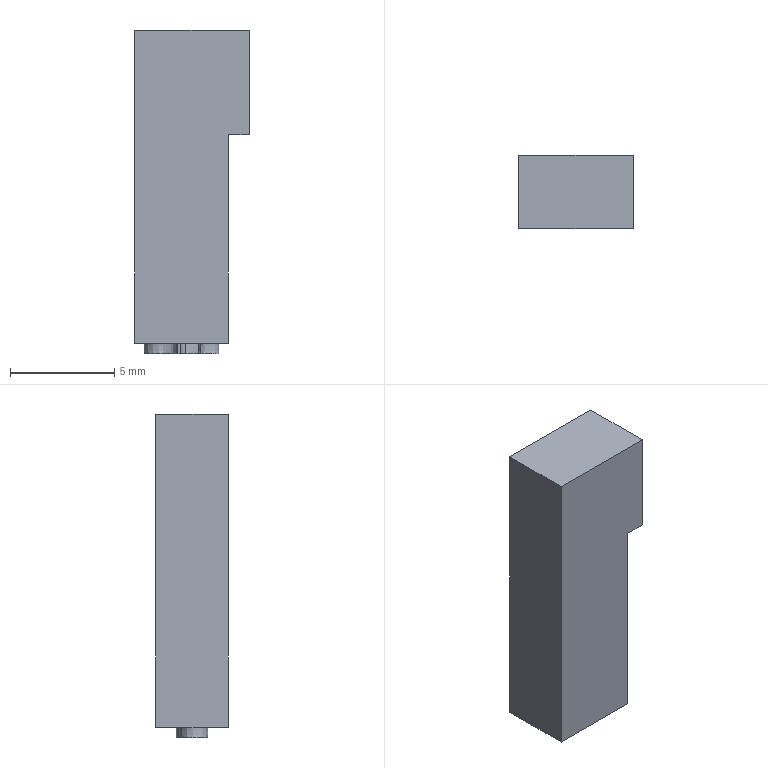Part | STEP file | gslz 2016.10.28-10_id1646_x_t | 1 solid | 24 faces | box 5.5 x 3.5 x 15.5 mm | volume 254.495 mm3 | other 14 | plane 10